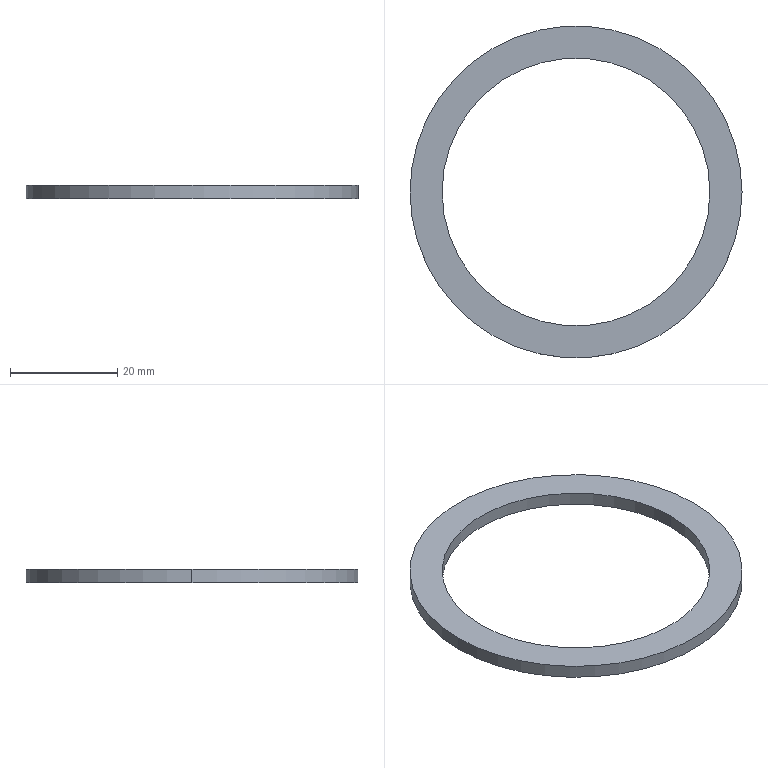Part | STEP file | Retaining ring SGN-4-13 | 1 solid | 6 faces | box 62 x 62 x 2.5 mm | volume 2639 mm3 | cylinder 4 | plane 2 | commonest cylinder face diameters 50 x2 62 x2
STEP:
#1=CARTESIAN_POINT('',(0.,0.,0.));
#2=DIRECTION('',(0.,0.,1.));
#3=DIRECTION('',(1.,0.,0.));
#4=AXIS2_PLACEMENT_3D('',#1,#2,#3);
#5=CARTESIAN_POINT('',(-25.,0.,2.5));
#6=VERTEX_POINT('',#5);
#7=CARTESIAN_POINT('',(-25.,0.,0.));
#8=VERTEX_POINT('',#7);
#9=CARTESIAN_POINT('',(-25.,0.,2.5));
#10=DIRECTION('',(0.,0.,-1.));
#11=VECTOR('',#10,1.);
#12=LINE('',#9,#11);
#13=CARTESIAN_POINT('',(0.,0.,2.5));
#14=DIRECTION('',(0.,0.,-1.));
#15=DIRECTION('',(-1.,0.,0.));
#16=AXIS2_PLACEMENT_3D('',#13,#14,#15);
#17=CYLINDRICAL_SURFACE('',#16,25.);
#18=CARTESIAN_POINT('',(6.283,0.));
#19=DIRECTION('',(0.,1.));
#20=VECTOR('',#19,1.);
#21=LINE('',#18,#20);
#22=(GEOMETRIC_REPRESENTATION_CONTEXT(2)PARAMETRIC_REPRESENTATION_CONTEXT()REPRESENTATION_CONTEXT('',''));
#23=DEFINITIONAL_REPRESENTATION('',(#21),#22);
#24=PCURVE('',#17,#23);
#25=CARTESIAN_POINT('',(0.,0.,2.5));
#26=DIRECTION('',(0.,0.,-1.));
#27=DIRECTION('',(-1.,0.,0.));
#28=AXIS2_PLACEMENT_3D('',#25,#26,#27);
#29=CYLINDRICAL_SURFACE('',#28,25.);
#30=CARTESIAN_POINT('',(0.,0.));
#31=DIRECTION('',(0.,1.));
#32=VECTOR('',#31,1.);
#33=LINE('',#30,#32);
#34=(GEOMETRIC_REPRESENTATION_CONTEXT(2)PARAMETRIC_REPRESENTATION_CONTEXT()REPRESENTATION_CONTEXT('',''));
#35=DEFINITIONAL_REPRESENTATION('',(#33),#34);
#36=PCURVE('',#29,#35);
#37=SURFACE_CURVE('',#12,(#24,#36),.PCURVE_S1.);
#38=EDGE_CURVE('',#6,#8,#37,.T.);
#39=ORIENTED_EDGE('',*,*,#38,.T.);
#40=CARTESIAN_POINT('',(25.,0.,0.));
#41=VERTEX_POINT('',#40);
#42=CARTESIAN_POINT('',(0.,0.,0.));
#43=DIRECTION('',(0.,0.,1.));
#44=DIRECTION('',(1.,0.,0.));
#45=AXIS2_PLACEMENT_3D('',#42,#43,#44);
#46=CIRCLE('',#45,25.);
#47=CARTESIAN_POINT('',(9.425,2.5));
#48=DIRECTION('',(-1.,0.));
#49=VECTOR('',#48,1.);
#50=LINE('',#47,#49);
#51=(GEOMETRIC_REPRESENTATION_CONTEXT(2)PARAMETRIC_REPRESENTATION_CONTEXT()REPRESENTATION_CONTEXT('',''));
#52=DEFINITIONAL_REPRESENTATION('',(#50),#51);
#53=PCURVE('',#17,#52);
#54=CARTESIAN_POINT('',(0.,0.,0.));
#55=DIRECTION('',(0.,0.,1.));
#56=DIRECTION('',(1.,0.,0.));
#57=AXIS2_PLACEMENT_3D('',#54,#55,#56);
#58=PLANE('',#57);
#59=CARTESIAN_POINT('',(0.,0.));
#60=DIRECTION('',(1.,0.));
#61=AXIS2_PLACEMENT_2D('',#59,#60);
#62=CIRCLE('',#61,25.);
#63=(GEOMETRIC_REPRESENTATION_CONTEXT(2)PARAMETRIC_REPRESENTATION_CONTEXT()REPRESENTATION_CONTEXT('',''));
#64=DEFINITIONAL_REPRESENTATION('',(#62),#63);
#65=PCURVE('',#58,#64);
#66=SURFACE_CURVE('',#46,(#53,#65),.PCURVE_S1.);
#67=EDGE_CURVE('',#8,#41,#66,.T.);
#68=ORIENTED_EDGE('',*,*,#67,.T.);
#69=CARTESIAN_POINT('',(25.,0.,2.5));
#70=VERTEX_POINT('',#69);
#71=CARTESIAN_POINT('',(25.,0.,2.5));
#72=DIRECTION('',(0.,0.,-1.));
#73=VECTOR('',#72,1.);
#74=LINE('',#71,#73);
#75=CARTESIAN_POINT('',(3.142,0.));
#76=DIRECTION('',(0.,1.));
#77=VECTOR('',#76,1.);
#78=LINE('',#75,#77);
#79=(GEOMETRIC_REPRESENTATION_CONTEXT(2)PARAMETRIC_REPRESENTATION_CONTEXT()REPRESENTATION_CONTEXT('',''));
#80=DEFINITIONAL_REPRESENTATION('',(#78),#79);
#81=PCURVE('',#17,#80);
#82=CARTESIAN_POINT('',(3.142,0.));
#83=DIRECTION('',(0.,1.));
#84=VECTOR('',#83,1.);
#85=LINE('',#82,#84);
#86=(GEOMETRIC_REPRESENTATION_CONTEXT(2)PARAMETRIC_REPRESENTATION_CONTEXT()REPRESENTATION_CONTEXT('',''));
#87=DEFINITIONAL_REPRESENTATION('',(#85),#86);
#88=PCURVE('',#29,#87);
#89=SURFACE_CURVE('',#74,(#81,#88),.PCURVE_S1.);
#90=EDGE_CURVE('',#70,#41,#89,.T.);
#91=ORIENTED_EDGE('',*,*,#90,.F.);
#92=CARTESIAN_POINT('',(0.,0.,2.5));
#93=DIRECTION('',(0.,0.,1.));
#94=DIRECTION('',(1.,0.,0.));
#95=AXIS2_PLACEMENT_3D('',#92,#93,#94);
#96=CIRCLE('',#95,25.);
#97=CARTESIAN_POINT('',(9.425,0.));
#98=DIRECTION('',(-1.,0.));
#99=VECTOR('',#98,1.);
#100=LINE('',#97,#99);
#101=(GEOMETRIC_REPRESENTATION_CONTEXT(2)PARAMETRIC_REPRESENTATION_CONTEXT()REPRESENTATION_CONTEXT('',''));
#102=DEFINITIONAL_REPRESENTATION('',(#100),#101);
#103=PCURVE('',#17,#102);
#104=CARTESIAN_POINT('',(0.,0.,2.5));
#105=DIRECTION('',(0.,0.,1.));
#106=DIRECTION('',(1.,0.,0.));
#107=AXIS2_PLACEMENT_3D('',#104,#105,#106);
#108=PLANE('',#107);
#109=CARTESIAN_POINT('',(0.,0.));
#110=DIRECTION('',(1.,0.));
#111=AXIS2_PLACEMENT_2D('',#109,#110);
#112=CIRCLE('',#111,25.);
#113=(GEOMETRIC_REPRESENTATION_CONTEXT(2)PARAMETRIC_REPRESENTATION_CONTEXT()REPRESENTATION_CONTEXT('',''));
#114=DEFINITIONAL_REPRESENTATION('',(#112),#113);
#115=PCURVE('',#108,#114);
#116=SURFACE_CURVE('',#96,(#103,#115),.PCURVE_S1.);
#117=EDGE_CURVE('',#6,#70,#116,.T.);
#118=ORIENTED_EDGE('',*,*,#117,.F.);
#119=EDGE_LOOP('',(#39,#68,#91,#118));
#120=FACE_BOUND('',#119,.F.);
#121=ADVANCED_FACE('',(#120),#17,.F.);
#122=CARTESIAN_POINT('',(31.,0.,2.5));
#123=VERTEX_POINT('',#122);
#124=CARTESIAN_POINT('',(-31.,0.,2.5));
#125=VERTEX_POINT('',#124);
#126=CARTESIAN_POINT('',(0.,0.,2.5));
#127=DIRECTION('',(0.,0.,1.));
#128=DIRECTION('',(1.,0.,0.));
#129=AXIS2_PLACEMENT_3D('',#126,#127,#128);
#130=CIRCLE('',#129,31.);
#131=CARTESIAN_POINT('',(0.,0.,2.5));
#132=DIRECTION('',(0.,0.,-1.));
#133=DIRECTION('',(-1.,0.,0.));
#134=AXIS2_PLACEMENT_3D('',#131,#132,#133);
#135=CYLINDRICAL_SURFACE('',#134,31.);
#136=CARTESIAN_POINT('',(3.142,0.));
#137=DIRECTION('',(-1.,0.));
#138=VECTOR('',#137,1.);
#139=LINE('',#136,#138);
#140=(GEOMETRIC_REPRESENTATION_CONTEXT(2)PARAMETRIC_REPRESENTATION_CONTEXT()REPRESENTATION_CONTEXT('',''));
#141=DEFINITIONAL_REPRESENTATION('',(#139),#140);
#142=PCURVE('',#135,#141);
#143=CARTESIAN_POINT('',(0.,0.));
#144=DIRECTION('',(1.,0.));
#145=AXIS2_PLACEMENT_2D('',#143,#144);
#146=CIRCLE('',#145,31.);
#147=(GEOMETRIC_REPRESENTATION_CONTEXT(2)PARAMETRIC_REPRESENTATION_CONTEXT()REPRESENTATION_CONTEXT('',''));
#148=DEFINITIONAL_REPRESENTATION('',(#146),#147);
#149=PCURVE('',#108,#148);
#150=SURFACE_CURVE('',#130,(#142,#149),.PCURVE_S1.);
#151=EDGE_CURVE('',#123,#125,#150,.T.);
#152=ORIENTED_EDGE('',*,*,#151,.F.);
#153=CARTESIAN_POINT('',(31.,0.,0.));
#154=VERTEX_POINT('',#153);
#155=CARTESIAN_POINT('',(31.,0.,2.5));
#156=DIRECTION('',(0.,0.,-1.));
#157=VECTOR('',#156,1.);
#158=LINE('',#155,#157);
#159=CARTESIAN_POINT('',(3.142,0.));
#160=DIRECTION('',(0.,1.));
#161=VECTOR('',#160,1.);
#162=LINE('',#159,#161);
#163=(GEOMETRIC_REPRESENTATION_CONTEXT(2)PARAMETRIC_REPRESENTATION_CONTEXT()REPRESENTATION_CONTEXT('',''));
#164=DEFINITIONAL_REPRESENTATION('',(#162),#163);
#165=PCURVE('',#135,#164);
#166=CARTESIAN_POINT('',(0.,0.,2.5));
#167=DIRECTION('',(0.,0.,-1.));
#168=DIRECTION('',(-1.,0.,0.));
#169=AXIS2_PLACEMENT_3D('',#166,#167,#168);
#170=CYLINDRICAL_SURFACE('',#169,31.);
#171=CARTESIAN_POINT('',(3.142,0.));
#172=DIRECTION('',(0.,1.));
#173=VECTOR('',#172,1.);
#174=LINE('',#171,#173);
#175=(GEOMETRIC_REPRESENTATION_CONTEXT(2)PARAMETRIC_REPRESENTATION_CONTEXT()REPRESENTATION_CONTEXT('',''));
#176=DEFINITIONAL_REPRESENTATION('',(#174),#175);
#177=PCURVE('',#170,#176);
#178=SURFACE_CURVE('',#158,(#165,#177),.PCURVE_S1.);
#179=EDGE_CURVE('',#123,#154,#178,.T.);
#180=ORIENTED_EDGE('',*,*,#179,.T.);
#181=CARTESIAN_POINT('',(-31.,0.,0.));
#182=VERTEX_POINT('',#181);
#183=CARTESIAN_POINT('',(0.,0.,0.));
#184=DIRECTION('',(0.,0.,1.));
#185=DIRECTION('',(1.,0.,0.));
#186=AXIS2_PLACEMENT_3D('',#183,#184,#185);
#187=CIRCLE('',#186,31.);
#188=CARTESIAN_POINT('',(3.142,2.5));
#189=DIRECTION('',(-1.,0.));
#190=VECTOR('',#189,1.);
#191=LINE('',#188,#190);
#192=(GEOMETRIC_REPRESENTATION_CONTEXT(2)PARAMETRIC_REPRESENTATION_CONTEXT()REPRESENTATION_CONTEXT('',''));
#193=DEFINITIONAL_REPRESENTATION('',(#191),#192);
#194=PCURVE('',#135,#193);
#195=CARTESIAN_POINT('',(0.,0.));
#196=DIRECTION('',(1.,0.));
#197=AXIS2_PLACEMENT_2D('',#195,#196);
#198=CIRCLE('',#197,31.);
#199=(GEOMETRIC_REPRESENTATION_CONTEXT(2)PARAMETRIC_REPRESENTATION_CONTEXT()REPRESENTATION_CONTEXT('',''));
#200=DEFINITIONAL_REPRESENTATION('',(#198),#199);
#201=PCURVE('',#58,#200);
#202=SURFACE_CURVE('',#187,(#194,#201),.PCURVE_S1.);
#203=EDGE_CURVE('',#154,#182,#202,.T.);
#204=ORIENTED_EDGE('',*,*,#203,.T.);
#205=CARTESIAN_POINT('',(-31.,0.,2.5));
#206=DIRECTION('',(0.,0.,-1.));
#207=VECTOR('',#206,1.);
#208=LINE('',#205,#207);
#209=CARTESIAN_POINT('',(0.,0.));
#210=DIRECTION('',(0.,1.));
#211=VECTOR('',#210,1.);
#212=LINE('',#209,#211);
#213=(GEOMETRIC_REPRESENTATION_CONTEXT(2)PARAMETRIC_REPRESENTATION_CONTEXT()REPRESENTATION_CONTEXT('',''));
#214=DEFINITIONAL_REPRESENTATION('',(#212),#213);
#215=PCURVE('',#135,#214);
#216=CARTESIAN_POINT('',(6.283,0.));
#217=DIRECTION('',(0.,1.));
#218=VECTOR('',#217,1.);
#219=LINE('',#216,#218);
#220=(GEOMETRIC_REPRESENTATION_CONTEXT(2)PARAMETRIC_REPRESENTATION_CONTEXT()REPRESENTATION_CONTEXT('',''));
#221=DEFINITIONAL_REPRESENTATION('',(#219),#220);
#222=PCURVE('',#170,#221);
#223=SURFACE_CURVE('',#208,(#215,#222),.PCURVE_S1.);
#224=EDGE_CURVE('',#125,#182,#223,.T.);
#225=ORIENTED_EDGE('',*,*,#224,.F.);
#226=EDGE_LOOP('',(#152,#180,#204,#225));
#227=FACE_BOUND('',#226,.T.);
#228=ADVANCED_FACE('',(#227),#135,.T.);
#229=CARTESIAN_POINT('',(0.,0.,2.5));
#230=DIRECTION('',(0.,0.,1.));
#231=DIRECTION('',(1.,0.,0.));
#232=AXIS2_PLACEMENT_3D('',#229,#230,#231);
#233=CIRCLE('',#232,31.);
#234=CARTESIAN_POINT('',(0.,0.));
#235=DIRECTION('',(1.,0.));
#236=AXIS2_PLACEMENT_2D('',#234,#235);
#237=CIRCLE('',#236,31.);
#238=(GEOMETRIC_REPRESENTATION_CONTEXT(2)PARAMETRIC_REPRESENTATION_CONTEXT()REPRESENTATION_CONTEXT('',''));
#239=DEFINITIONAL_REPRESENTATION('',(#237),#238);
#240=PCURVE('',#108,#239);
#241=CARTESIAN_POINT('',(9.425,0.));
#242=DIRECTION('',(-1.,0.));
#243=VECTOR('',#242,1.);
#244=LINE('',#241,#243);
#245=(GEOMETRIC_REPRESENTATION_CONTEXT(2)PARAMETRIC_REPRESENTATION_CONTEXT()REPRESENTATION_CONTEXT('',''));
#246=DEFINITIONAL_REPRESENTATION('',(#244),#245);
#247=PCURVE('',#170,#246);
#248=SURFACE_CURVE('',#233,(#240,#247),.PCURVE_S1.);
#249=EDGE_CURVE('',#125,#123,#248,.T.);
#250=ORIENTED_EDGE('',*,*,#249,.T.);
#251=ORIENTED_EDGE('',*,*,#151,.T.);
#252=EDGE_LOOP('',(#250,#251));
#253=FACE_BOUND('',#252,.T.);
#254=ORIENTED_EDGE('',*,*,#117,.F.);
#255=CARTESIAN_POINT('',(0.,0.,2.5));
#256=DIRECTION('',(0.,0.,1.));
#257=DIRECTION('',(1.,0.,0.));
#258=AXIS2_PLACEMENT_3D('',#255,#256,#257);
#259=CIRCLE('',#258,25.);
#260=CARTESIAN_POINT('',(0.,0.));
#261=DIRECTION('',(1.,0.));
#262=AXIS2_PLACEMENT_2D('',#260,#261);
#263=CIRCLE('',#262,25.);
#264=(GEOMETRIC_REPRESENTATION_CONTEXT(2)PARAMETRIC_REPRESENTATION_CONTEXT()REPRESENTATION_CONTEXT('',''));
#265=DEFINITIONAL_REPRESENTATION('',(#263),#264);
#266=PCURVE('',#108,#265);
#267=CARTESIAN_POINT('',(3.142,0.));
#268=DIRECTION('',(-1.,0.));
#269=VECTOR('',#268,1.);
#270=LINE('',#267,#269);
#271=(GEOMETRIC_REPRESENTATION_CONTEXT(2)PARAMETRIC_REPRESENTATION_CONTEXT()REPRESENTATION_CONTEXT('',''));
#272=DEFINITIONAL_REPRESENTATION('',(#270),#271);
#273=PCURVE('',#29,#272);
#274=SURFACE_CURVE('',#259,(#266,#273),.PCURVE_S1.);
#275=EDGE_CURVE('',#70,#6,#274,.T.);
#276=ORIENTED_EDGE('',*,*,#275,.F.);
#277=EDGE_LOOP('',(#254,#276));
#278=FACE_BOUND('',#277,.T.);
#279=ADVANCED_FACE('',(#253,#278),#108,.T.);
#280=CARTESIAN_POINT('',(0.,0.,0.));
#281=DIRECTION('',(0.,0.,1.));
#282=DIRECTION('',(1.,0.,0.));
#283=AXIS2_PLACEMENT_3D('',#280,#281,#282);
#284=CIRCLE('',#283,31.);
#285=CARTESIAN_POINT('',(0.,0.));
#286=DIRECTION('',(1.,0.));
#287=AXIS2_PLACEMENT_2D('',#285,#286);
#288=CIRCLE('',#287,31.);
#289=(GEOMETRIC_REPRESENTATION_CONTEXT(2)PARAMETRIC_REPRESENTATION_CONTEXT()REPRESENTATION_CONTEXT('',''));
#290=DEFINITIONAL_REPRESENTATION('',(#288),#289);
#291=PCURVE('',#58,#290);
#292=CARTESIAN_POINT('',(9.425,2.5));
#293=DIRECTION('',(-1.,0.));
#294=VECTOR('',#293,1.);
#295=LINE('',#292,#294);
#296=(GEOMETRIC_REPRESENTATION_CONTEXT(2)PARAMETRIC_REPRESENTATION_CONTEXT()REPRESENTATION_CONTEXT('',''));
#297=DEFINITIONAL_REPRESENTATION('',(#295),#296);
#298=PCURVE('',#170,#297);
#299=SURFACE_CURVE('',#284,(#291,#298),.PCURVE_S1.);
#300=EDGE_CURVE('',#182,#154,#299,.T.);
#301=ORIENTED_EDGE('',*,*,#300,.F.);
#302=ORIENTED_EDGE('',*,*,#203,.F.);
#303=EDGE_LOOP('',(#301,#302));
#304=FACE_BOUND('',#303,.T.);
#305=ORIENTED_EDGE('',*,*,#67,.T.);
#306=CARTESIAN_POINT('',(0.,0.,0.));
#307=DIRECTION('',(0.,0.,1.));
#308=DIRECTION('',(1.,0.,0.));
#309=AXIS2_PLACEMENT_3D('',#306,#307,#308);
#310=CIRCLE('',#309,25.);
#311=CARTESIAN_POINT('',(0.,0.));
#312=DIRECTION('',(1.,0.));
#313=AXIS2_PLACEMENT_2D('',#311,#312);
#314=CIRCLE('',#313,25.);
#315=(GEOMETRIC_REPRESENTATION_CONTEXT(2)PARAMETRIC_REPRESENTATION_CONTEXT()REPRESENTATION_CONTEXT('',''));
#316=DEFINITIONAL_REPRESENTATION('',(#314),#315);
#317=PCURVE('',#58,#316);
#318=CARTESIAN_POINT('',(3.142,2.5));
#319=DIRECTION('',(-1.,0.));
#320=VECTOR('',#319,1.);
#321=LINE('',#318,#320);
#322=(GEOMETRIC_REPRESENTATION_CONTEXT(2)PARAMETRIC_REPRESENTATION_CONTEXT()REPRESENTATION_CONTEXT('',''));
#323=DEFINITIONAL_REPRESENTATION('',(#321),#322);
#324=PCURVE('',#29,#323);
#325=SURFACE_CURVE('',#310,(#317,#324),.PCURVE_S1.);
#326=EDGE_CURVE('',#41,#8,#325,.T.);
#327=ORIENTED_EDGE('',*,*,#326,.T.);
#328=EDGE_LOOP('',(#305,#327));
#329=FACE_BOUND('',#328,.T.);
#330=ADVANCED_FACE('',(#304,#329),#58,.F.);
#331=ORIENTED_EDGE('',*,*,#179,.F.);
#332=ORIENTED_EDGE('',*,*,#249,.F.);
#333=ORIENTED_EDGE('',*,*,#224,.T.);
#334=ORIENTED_EDGE('',*,*,#300,.T.);
#335=EDGE_LOOP('',(#331,#332,#333,#334));
#336=FACE_BOUND('',#335,.T.);
#337=ADVANCED_FACE('',(#336),#170,.T.);
#338=ORIENTED_EDGE('',*,*,#326,.T.);
#339=ORIENTED_EDGE('',*,*,#38,.F.);
#340=ORIENTED_EDGE('',*,*,#275,.F.);
#341=ORIENTED_EDGE('',*,*,#90,.T.);
#342=EDGE_LOOP('',(#338,#339,#340,#341));
#343=FACE_BOUND('',#342,.F.);
#344=ADVANCED_FACE('',(#343),#29,.F.);
#345=CLOSED_SHELL('',(#121,#228,#279,#330,#337,#344));
#346=MANIFOLD_SOLID_BREP('',#345);
#347=(LENGTH_UNIT()NAMED_UNIT(*)SI_UNIT(.MILLI.,.METRE.));
#348=UNCERTAINTY_MEASURE_WITH_UNIT(LENGTH_MEASURE(0.0000001),#347,'','');
#349=(NAMED_UNIT(*)PLANE_ANGLE_UNIT()SI_UNIT($,.RADIAN.));
#350=(NAMED_UNIT(*)SI_UNIT($,.STERADIAN.)SOLID_ANGLE_UNIT());
#351=(GEOMETRIC_REPRESENTATION_CONTEXT(3)GLOBAL_UNCERTAINTY_ASSIGNED_CONTEXT((#348))GLOBAL_UNIT_ASSIGNED_CONTEXT((#347,#349,#350))REPRESENTATION_CONTEXT('',''));
#352=ADVANCED_BREP_SHAPE_REPRESENTATION('',(#4,#346),#351);